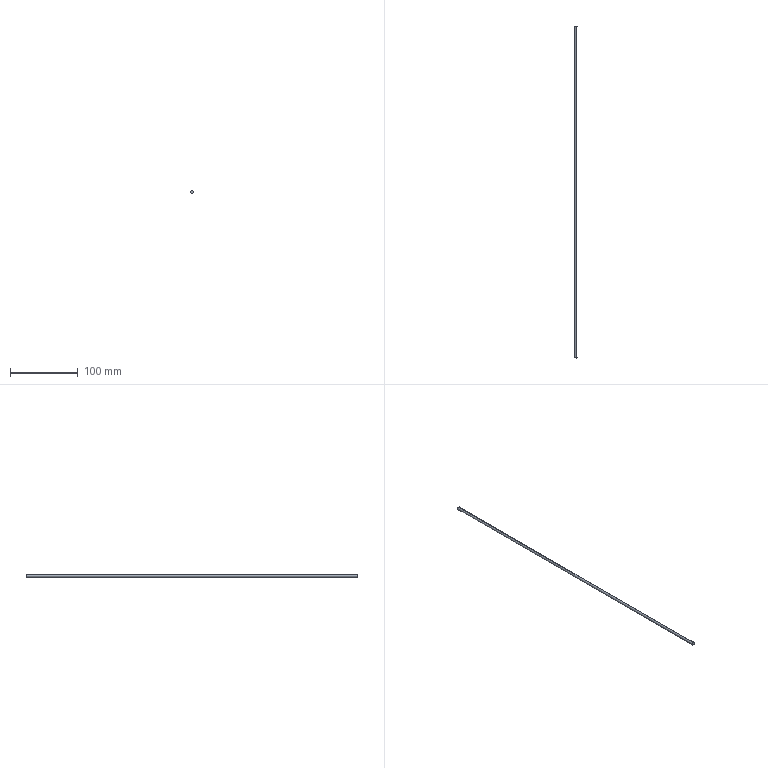Part | STEP file | Gear shaft | 1 solid | 4 faces | box 4 x 491 x 4 mm | volume 6170 mm3 | cylinder 2 | plane 2 | commonest cylinder face diameters 4 x2
STEP:
#1=CARTESIAN_POINT('',(0.,0.,0.));
#2=DIRECTION('',(0.,0.,1.));
#3=DIRECTION('',(1.,0.,0.));
#4=AXIS2_PLACEMENT_3D('',#1,#2,#3);
#5=CARTESIAN_POINT('',(0.,491.,2.));
#6=VERTEX_POINT('',#5);
#7=CARTESIAN_POINT('',(0.,491.,-2.));
#8=VERTEX_POINT('',#7);
#9=CARTESIAN_POINT('',(0.,491.,0.));
#10=DIRECTION('',(0.,1.,0.));
#11=DIRECTION('',(0.,0.,1.));
#12=AXIS2_PLACEMENT_3D('',#9,#10,#11);
#13=CIRCLE('',#12,2.);
#14=CARTESIAN_POINT('',(0.,491.,0.));
#15=DIRECTION('',(0.,-1.,0.));
#16=DIRECTION('',(0.,0.,-1.));
#17=AXIS2_PLACEMENT_3D('',#14,#15,#16);
#18=CYLINDRICAL_SURFACE('',#17,2.);
#19=CARTESIAN_POINT('',(3.142,0.));
#20=DIRECTION('',(-1.,0.));
#21=VECTOR('',#20,1.);
#22=LINE('',#19,#21);
#23=(GEOMETRIC_REPRESENTATION_CONTEXT(2)PARAMETRIC_REPRESENTATION_CONTEXT()REPRESENTATION_CONTEXT('',''));
#24=DEFINITIONAL_REPRESENTATION('',(#22),#23);
#25=PCURVE('',#18,#24);
#26=CARTESIAN_POINT('',(0.,491.,0.));
#27=DIRECTION('',(0.,1.,0.));
#28=DIRECTION('',(0.,0.,1.));
#29=AXIS2_PLACEMENT_3D('',#26,#27,#28);
#30=PLANE('',#29);
#31=CARTESIAN_POINT('',(0.,0.));
#32=DIRECTION('',(1.,0.));
#33=AXIS2_PLACEMENT_2D('',#31,#32);
#34=CIRCLE('',#33,2.);
#35=(GEOMETRIC_REPRESENTATION_CONTEXT(2)PARAMETRIC_REPRESENTATION_CONTEXT()REPRESENTATION_CONTEXT('',''));
#36=DEFINITIONAL_REPRESENTATION('',(#34),#35);
#37=PCURVE('',#30,#36);
#38=SURFACE_CURVE('',#13,(#25,#37),.PCURVE_S1.);
#39=EDGE_CURVE('',#6,#8,#38,.T.);
#40=ORIENTED_EDGE('',*,*,#39,.F.);
#41=CARTESIAN_POINT('',(0.,0.,2.));
#42=VERTEX_POINT('',#41);
#43=CARTESIAN_POINT('',(0.,491.,2.));
#44=DIRECTION('',(0.,-1.,0.));
#45=VECTOR('',#44,1.);
#46=LINE('',#43,#45);
#47=CARTESIAN_POINT('',(3.142,0.));
#48=DIRECTION('',(0.,1.));
#49=VECTOR('',#48,1.);
#50=LINE('',#47,#49);
#51=(GEOMETRIC_REPRESENTATION_CONTEXT(2)PARAMETRIC_REPRESENTATION_CONTEXT()REPRESENTATION_CONTEXT('',''));
#52=DEFINITIONAL_REPRESENTATION('',(#50),#51);
#53=PCURVE('',#18,#52);
#54=CARTESIAN_POINT('',(0.,491.,0.));
#55=DIRECTION('',(0.,-1.,0.));
#56=DIRECTION('',(0.,0.,-1.));
#57=AXIS2_PLACEMENT_3D('',#54,#55,#56);
#58=CYLINDRICAL_SURFACE('',#57,2.);
#59=CARTESIAN_POINT('',(3.142,0.));
#60=DIRECTION('',(0.,1.));
#61=VECTOR('',#60,1.);
#62=LINE('',#59,#61);
#63=(GEOMETRIC_REPRESENTATION_CONTEXT(2)PARAMETRIC_REPRESENTATION_CONTEXT()REPRESENTATION_CONTEXT('',''));
#64=DEFINITIONAL_REPRESENTATION('',(#62),#63);
#65=PCURVE('',#58,#64);
#66=SURFACE_CURVE('',#46,(#53,#65),.PCURVE_S1.);
#67=EDGE_CURVE('',#6,#42,#66,.T.);
#68=ORIENTED_EDGE('',*,*,#67,.T.);
#69=CARTESIAN_POINT('',(0.,0.,-2.));
#70=VERTEX_POINT('',#69);
#71=CARTESIAN_POINT('',(0.,0.,0.));
#72=DIRECTION('',(0.,1.,0.));
#73=DIRECTION('',(0.,0.,1.));
#74=AXIS2_PLACEMENT_3D('',#71,#72,#73);
#75=CIRCLE('',#74,2.);
#76=CARTESIAN_POINT('',(3.142,491.));
#77=DIRECTION('',(-1.,0.));
#78=VECTOR('',#77,1.);
#79=LINE('',#76,#78);
#80=(GEOMETRIC_REPRESENTATION_CONTEXT(2)PARAMETRIC_REPRESENTATION_CONTEXT()REPRESENTATION_CONTEXT('',''));
#81=DEFINITIONAL_REPRESENTATION('',(#79),#80);
#82=PCURVE('',#18,#81);
#83=CARTESIAN_POINT('',(0.,0.,0.));
#84=DIRECTION('',(0.,1.,0.));
#85=DIRECTION('',(0.,0.,1.));
#86=AXIS2_PLACEMENT_3D('',#83,#84,#85);
#87=PLANE('',#86);
#88=CARTESIAN_POINT('',(0.,0.));
#89=DIRECTION('',(1.,0.));
#90=AXIS2_PLACEMENT_2D('',#88,#89);
#91=CIRCLE('',#90,2.);
#92=(GEOMETRIC_REPRESENTATION_CONTEXT(2)PARAMETRIC_REPRESENTATION_CONTEXT()REPRESENTATION_CONTEXT('',''));
#93=DEFINITIONAL_REPRESENTATION('',(#91),#92);
#94=PCURVE('',#87,#93);
#95=SURFACE_CURVE('',#75,(#82,#94),.PCURVE_S1.);
#96=EDGE_CURVE('',#42,#70,#95,.T.);
#97=ORIENTED_EDGE('',*,*,#96,.T.);
#98=CARTESIAN_POINT('',(0.,491.,-2.));
#99=DIRECTION('',(0.,-1.,0.));
#100=VECTOR('',#99,1.);
#101=LINE('',#98,#100);
#102=CARTESIAN_POINT('',(0.,0.));
#103=DIRECTION('',(0.,1.));
#104=VECTOR('',#103,1.);
#105=LINE('',#102,#104);
#106=(GEOMETRIC_REPRESENTATION_CONTEXT(2)PARAMETRIC_REPRESENTATION_CONTEXT()REPRESENTATION_CONTEXT('',''));
#107=DEFINITIONAL_REPRESENTATION('',(#105),#106);
#108=PCURVE('',#18,#107);
#109=CARTESIAN_POINT('',(6.283,0.));
#110=DIRECTION('',(0.,1.));
#111=VECTOR('',#110,1.);
#112=LINE('',#109,#111);
#113=(GEOMETRIC_REPRESENTATION_CONTEXT(2)PARAMETRIC_REPRESENTATION_CONTEXT()REPRESENTATION_CONTEXT('',''));
#114=DEFINITIONAL_REPRESENTATION('',(#112),#113);
#115=PCURVE('',#58,#114);
#116=SURFACE_CURVE('',#101,(#108,#115),.PCURVE_S1.);
#117=EDGE_CURVE('',#8,#70,#116,.T.);
#118=ORIENTED_EDGE('',*,*,#117,.F.);
#119=EDGE_LOOP('',(#40,#68,#97,#118));
#120=FACE_BOUND('',#119,.T.);
#121=ADVANCED_FACE('',(#120),#18,.T.);
#122=ORIENTED_EDGE('',*,*,#67,.F.);
#123=CARTESIAN_POINT('',(0.,491.,0.));
#124=DIRECTION('',(0.,1.,0.));
#125=DIRECTION('',(0.,0.,1.));
#126=AXIS2_PLACEMENT_3D('',#123,#124,#125);
#127=CIRCLE('',#126,2.);
#128=CARTESIAN_POINT('',(9.425,0.));
#129=DIRECTION('',(-1.,0.));
#130=VECTOR('',#129,1.);
#131=LINE('',#128,#130);
#132=(GEOMETRIC_REPRESENTATION_CONTEXT(2)PARAMETRIC_REPRESENTATION_CONTEXT()REPRESENTATION_CONTEXT('',''));
#133=DEFINITIONAL_REPRESENTATION('',(#131),#132);
#134=PCURVE('',#58,#133);
#135=CARTESIAN_POINT('',(0.,0.));
#136=DIRECTION('',(1.,0.));
#137=AXIS2_PLACEMENT_2D('',#135,#136);
#138=CIRCLE('',#137,2.);
#139=(GEOMETRIC_REPRESENTATION_CONTEXT(2)PARAMETRIC_REPRESENTATION_CONTEXT()REPRESENTATION_CONTEXT('',''));
#140=DEFINITIONAL_REPRESENTATION('',(#138),#139);
#141=PCURVE('',#30,#140);
#142=SURFACE_CURVE('',#127,(#134,#141),.PCURVE_S1.);
#143=EDGE_CURVE('',#8,#6,#142,.T.);
#144=ORIENTED_EDGE('',*,*,#143,.F.);
#145=ORIENTED_EDGE('',*,*,#117,.T.);
#146=CARTESIAN_POINT('',(0.,0.,0.));
#147=DIRECTION('',(0.,1.,0.));
#148=DIRECTION('',(0.,0.,1.));
#149=AXIS2_PLACEMENT_3D('',#146,#147,#148);
#150=CIRCLE('',#149,2.);
#151=CARTESIAN_POINT('',(9.425,491.));
#152=DIRECTION('',(-1.,0.));
#153=VECTOR('',#152,1.);
#154=LINE('',#151,#153);
#155=(GEOMETRIC_REPRESENTATION_CONTEXT(2)PARAMETRIC_REPRESENTATION_CONTEXT()REPRESENTATION_CONTEXT('',''));
#156=DEFINITIONAL_REPRESENTATION('',(#154),#155);
#157=PCURVE('',#58,#156);
#158=CARTESIAN_POINT('',(0.,0.));
#159=DIRECTION('',(1.,0.));
#160=AXIS2_PLACEMENT_2D('',#158,#159);
#161=CIRCLE('',#160,2.);
#162=(GEOMETRIC_REPRESENTATION_CONTEXT(2)PARAMETRIC_REPRESENTATION_CONTEXT()REPRESENTATION_CONTEXT('',''));
#163=DEFINITIONAL_REPRESENTATION('',(#161),#162);
#164=PCURVE('',#87,#163);
#165=SURFACE_CURVE('',#150,(#157,#164),.PCURVE_S1.);
#166=EDGE_CURVE('',#70,#42,#165,.T.);
#167=ORIENTED_EDGE('',*,*,#166,.T.);
#168=EDGE_LOOP('',(#122,#144,#145,#167));
#169=FACE_BOUND('',#168,.T.);
#170=ADVANCED_FACE('',(#169),#58,.T.);
#171=ORIENTED_EDGE('',*,*,#143,.T.);
#172=ORIENTED_EDGE('',*,*,#39,.T.);
#173=EDGE_LOOP('',(#171,#172));
#174=FACE_BOUND('',#173,.T.);
#175=ADVANCED_FACE('',(#174),#30,.T.);
#176=ORIENTED_EDGE('',*,*,#166,.F.);
#177=ORIENTED_EDGE('',*,*,#96,.F.);
#178=EDGE_LOOP('',(#176,#177));
#179=FACE_BOUND('',#178,.T.);
#180=ADVANCED_FACE('',(#179),#87,.F.);
#181=CLOSED_SHELL('',(#121,#170,#175,#180));
#182=MANIFOLD_SOLID_BREP('',#181);
#183=(LENGTH_UNIT()NAMED_UNIT(*)SI_UNIT(.MILLI.,.METRE.));
#184=UNCERTAINTY_MEASURE_WITH_UNIT(LENGTH_MEASURE(0.0000001),#183,'','');
#185=(NAMED_UNIT(*)PLANE_ANGLE_UNIT()SI_UNIT($,.RADIAN.));
#186=(NAMED_UNIT(*)SI_UNIT($,.STERADIAN.)SOLID_ANGLE_UNIT());
#187=(GEOMETRIC_REPRESENTATION_CONTEXT(3)GLOBAL_UNCERTAINTY_ASSIGNED_CONTEXT((#184))GLOBAL_UNIT_ASSIGNED_CONTEXT((#183,#185,#186))REPRESENTATION_CONTEXT('',''));
#188=ADVANCED_BREP_SHAPE_REPRESENTATION('',(#4,#182),#187);